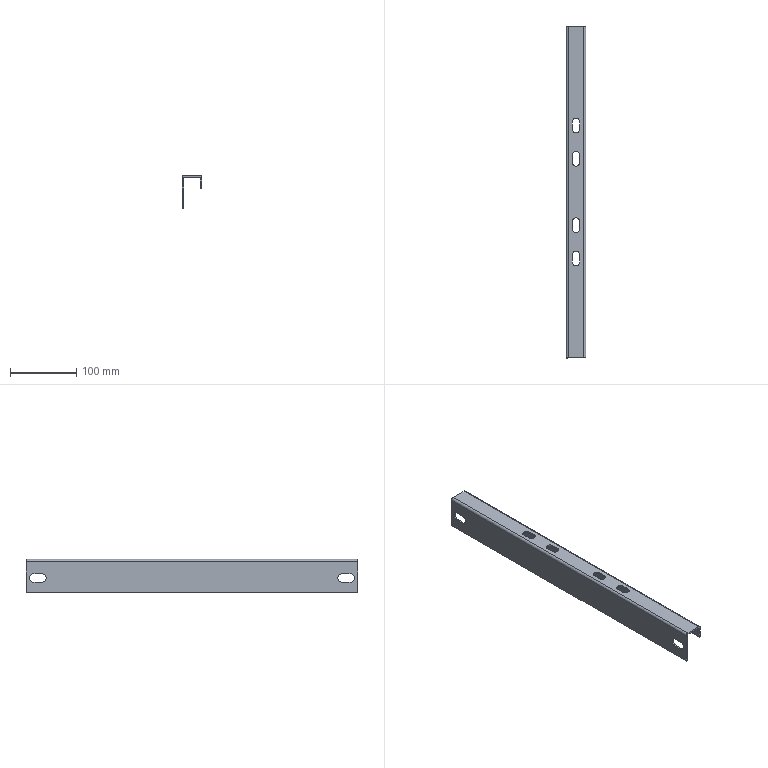Part | SolidWorks | features ICE 2, FlatPattern 1, SMBaseFlange 1, SheetMetal 1 | 1 solid | 46 faces | box 30 x 500 x 50 mm | volume 112732 mm3 | plane 30 | cylinder 16 | commonest cylinder face diameters 11 x8 13 x4 2 x2 7 x2
STEP:
#1=CARTESIAN_POINT('',(0.,250.,-3.5));
#2=VERTEX_POINT('',#1);
#3=CARTESIAN_POINT('',(2.5,250.,-3.5));
#4=VERTEX_POINT('',#3);
#5=CARTESIAN_POINT('',(0.,250.,-3.5));
#6=DIRECTION('',(1.,0.,0.));
#7=VECTOR('',#6,1000.);
#8=LINE('',#5,#7);
#9=EDGE_CURVE('',#2,#4,#8,.T.);
#10=ORIENTED_EDGE('',*,*,#9,.F.);
#11=CARTESIAN_POINT('',(3.5,250.,0.));
#12=VERTEX_POINT('',#11);
#13=CARTESIAN_POINT('',(3.5,250.,-3.5));
#14=DIRECTION('',(0.,1.,0.));
#15=DIRECTION('',(0.,0.,-1.));
#16=AXIS2_PLACEMENT_3D('',#13,#14,#15);
#17=CIRCLE('',#16,3.5);
#18=EDGE_CURVE('',#2,#12,#17,.T.);
#19=ORIENTED_EDGE('',*,*,#18,.T.);
#20=CARTESIAN_POINT('',(3.5,250.,-2.5));
#21=VERTEX_POINT('',#20);
#22=CARTESIAN_POINT('',(3.5,250.,-2.5));
#23=DIRECTION('',(0.,0.,1.));
#24=VECTOR('',#23,1000.);
#25=LINE('',#22,#24);
#26=EDGE_CURVE('',#21,#12,#25,.T.);
#27=ORIENTED_EDGE('',*,*,#26,.F.);
#28=CARTESIAN_POINT('',(3.5,250.,-3.5));
#29=DIRECTION('',(0.,1.,0.));
#30=DIRECTION('',(1.,0.,0.));
#31=AXIS2_PLACEMENT_3D('',#28,#29,#30);
#32=CIRCLE('',#31,1.);
#33=EDGE_CURVE('',#4,#21,#32,.T.);
#34=ORIENTED_EDGE('',*,*,#33,.F.);
#35=EDGE_LOOP('',(#10,#19,#27,#34));
#36=FACE_OUTER_BOUND('',#35,.T.);
#37=CARTESIAN_POINT('',(0.,250.,-3.5));
#38=DIRECTION('',(0.,1.,0.));
#39=DIRECTION('',(0.,0.,1.));
#40=AXIS2_PLACEMENT_3D('',#37,#38,#39);
#41=PLANE('',#40);
#42=ADVANCED_FACE('',(#36),#41,.T.);
#43=CARTESIAN_POINT('',(0.,250.,-50.));
#44=VERTEX_POINT('',#43);
#45=CARTESIAN_POINT('',(0.,250.,0.));
#46=DIRECTION('',(0.,0.,1.));
#47=VECTOR('',#46,1000.);
#48=LINE('',#45,#47);
#49=EDGE_CURVE('',#44,#2,#48,.T.);
#50=ORIENTED_EDGE('',*,*,#49,.T.);
#51=ORIENTED_EDGE('',*,*,#9,.T.);
#52=CARTESIAN_POINT('',(2.5,250.,-50.));
#53=VERTEX_POINT('',#52);
#54=CARTESIAN_POINT('',(2.5,250.,0.));
#55=DIRECTION('',(0.,0.,1.));
#56=VECTOR('',#55,1000.);
#57=LINE('',#54,#56);
#58=EDGE_CURVE('',#53,#4,#57,.T.);
#59=ORIENTED_EDGE('',*,*,#58,.F.);
#60=CARTESIAN_POINT('',(0.,250.,-50.));
#61=DIRECTION('',(1.,0.,0.));
#62=VECTOR('',#61,1000.);
#63=LINE('',#60,#62);
#64=EDGE_CURVE('',#44,#53,#63,.T.);
#65=ORIENTED_EDGE('',*,*,#64,.F.);
#66=EDGE_LOOP('',(#50,#51,#59,#65));
#67=FACE_OUTER_BOUND('',#66,.T.);
#68=CARTESIAN_POINT('',(3.5,250.,-2.5));
#69=DIRECTION('',(0.,1.,0.));
#70=DIRECTION('',(0.,0.,1.));
#71=AXIS2_PLACEMENT_3D('',#68,#69,#70);
#72=PLANE('',#71);
#73=ADVANCED_FACE('',(#67),#72,.T.);
#74=CARTESIAN_POINT('',(3.5,-250.,0.));
#75=VERTEX_POINT('',#74);
#76=CARTESIAN_POINT('',(3.5,-250.,-2.5));
#77=VERTEX_POINT('',#76);
#78=CARTESIAN_POINT('',(3.5,-250.,0.));
#79=DIRECTION('',(0.,0.,-1.));
#80=VECTOR('',#79,1000.);
#81=LINE('',#78,#80);
#82=EDGE_CURVE('',#75,#77,#81,.T.);
#83=ORIENTED_EDGE('',*,*,#82,.F.);
#84=CARTESIAN_POINT('',(0.,-250.,-3.5));
#85=VERTEX_POINT('',#84);
#86=CARTESIAN_POINT('',(3.5,-250.,-3.5));
#87=DIRECTION('',(0.,1.,0.));
#88=DIRECTION('',(0.,0.,-1.));
#89=AXIS2_PLACEMENT_3D('',#86,#87,#88);
#90=CIRCLE('',#89,3.5);
#91=EDGE_CURVE('',#85,#75,#90,.T.);
#92=ORIENTED_EDGE('',*,*,#91,.F.);
#93=CARTESIAN_POINT('',(2.5,-250.,-3.5));
#94=VERTEX_POINT('',#93);
#95=CARTESIAN_POINT('',(2.5,-250.,-3.5));
#96=DIRECTION('',(-1.,0.,0.));
#97=VECTOR('',#96,1000.);
#98=LINE('',#95,#97);
#99=EDGE_CURVE('',#94,#85,#98,.T.);
#100=ORIENTED_EDGE('',*,*,#99,.F.);
#101=CARTESIAN_POINT('',(3.5,-250.,-3.5));
#102=DIRECTION('',(0.,1.,0.));
#103=DIRECTION('',(1.,0.,0.));
#104=AXIS2_PLACEMENT_3D('',#101,#102,#103);
#105=CIRCLE('',#104,1.);
#106=EDGE_CURVE('',#94,#77,#105,.T.);
#107=ORIENTED_EDGE('',*,*,#106,.T.);
#108=EDGE_LOOP('',(#83,#92,#100,#107));
#109=FACE_OUTER_BOUND('',#108,.T.);
#110=CARTESIAN_POINT('',(3.5,-250.,0.));
#111=DIRECTION('',(0.,-1.,0.));
#112=DIRECTION('',(0.,0.,-1.));
#113=AXIS2_PLACEMENT_3D('',#110,#111,#112);
#114=PLANE('',#113);
#115=ADVANCED_FACE('',(#109),#114,.T.);
#116=CARTESIAN_POINT('',(26.5,-250.,0.));
#117=VERTEX_POINT('',#116);
#118=CARTESIAN_POINT('',(0.,-250.,0.));
#119=DIRECTION('',(1.,0.,0.));
#120=VECTOR('',#119,1000.);
#121=LINE('',#118,#120);
#122=EDGE_CURVE('',#75,#117,#121,.T.);
#123=ORIENTED_EDGE('',*,*,#122,.F.);
#124=ORIENTED_EDGE('',*,*,#82,.T.);
#125=CARTESIAN_POINT('',(26.5,-250.,-2.5));
#126=VERTEX_POINT('',#125);
#127=CARTESIAN_POINT('',(0.,-250.,-2.5));
#128=DIRECTION('',(1.,0.,0.));
#129=VECTOR('',#128,1000.);
#130=LINE('',#127,#129);
#131=EDGE_CURVE('',#77,#126,#130,.T.);
#132=ORIENTED_EDGE('',*,*,#131,.T.);
#133=CARTESIAN_POINT('',(26.5,-250.,-2.5));
#134=DIRECTION('',(0.,0.,1.));
#135=VECTOR('',#134,1000.);
#136=LINE('',#133,#135);
#137=EDGE_CURVE('',#126,#117,#136,.T.);
#138=ORIENTED_EDGE('',*,*,#137,.T.);
#139=EDGE_LOOP('',(#123,#124,#132,#138));
#140=FACE_OUTER_BOUND('',#139,.T.);
#141=CARTESIAN_POINT('',(2.5,-250.,-3.5));
#142=DIRECTION('',(0.,-1.,0.));
#143=DIRECTION('',(0.,0.,-1.));
#144=AXIS2_PLACEMENT_3D('',#141,#142,#143);
#145=PLANE('',#144);
#146=ADVANCED_FACE('',(#140),#145,.T.);
#147=CARTESIAN_POINT('',(26.5,250.,0.));
#148=VERTEX_POINT('',#147);
#149=CARTESIAN_POINT('',(26.5,250.,-2.5));
#150=VERTEX_POINT('',#149);
#151=CARTESIAN_POINT('',(26.5,250.,0.));
#152=DIRECTION('',(0.,0.,-1.));
#153=VECTOR('',#152,1000.);
#154=LINE('',#151,#153);
#155=EDGE_CURVE('',#148,#150,#154,.T.);
#156=ORIENTED_EDGE('',*,*,#155,.F.);
#157=CARTESIAN_POINT('',(30.,250.,-3.5));
#158=VERTEX_POINT('',#157);
#159=CARTESIAN_POINT('',(26.5,250.,-3.5));
#160=DIRECTION('',(0.,1.,0.));
#161=DIRECTION('',(0.,0.,-1.));
#162=AXIS2_PLACEMENT_3D('',#159,#160,#161);
#163=CIRCLE('',#162,3.5);
#164=EDGE_CURVE('',#148,#158,#163,.T.);
#165=ORIENTED_EDGE('',*,*,#164,.T.);
#166=CARTESIAN_POINT('',(27.5,250.,-3.5));
#167=VERTEX_POINT('',#166);
#168=CARTESIAN_POINT('',(27.5,250.,-3.5));
#169=DIRECTION('',(1.,0.,0.));
#170=VECTOR('',#169,1000.);
#171=LINE('',#168,#170);
#172=EDGE_CURVE('',#167,#158,#171,.T.);
#173=ORIENTED_EDGE('',*,*,#172,.F.);
#174=CARTESIAN_POINT('',(26.5,250.,-3.5));
#175=DIRECTION('',(0.,1.,0.));
#176=DIRECTION('',(1.,0.,0.));
#177=AXIS2_PLACEMENT_3D('',#174,#175,#176);
#178=CIRCLE('',#177,1.);
#179=EDGE_CURVE('',#150,#167,#178,.T.);
#180=ORIENTED_EDGE('',*,*,#179,.F.);
#181=EDGE_LOOP('',(#156,#165,#173,#180));
#182=FACE_OUTER_BOUND('',#181,.T.);
#183=CARTESIAN_POINT('',(26.5,250.,0.));
#184=DIRECTION('',(0.,1.,0.));
#185=DIRECTION('',(0.,0.,1.));
#186=AXIS2_PLACEMENT_3D('',#183,#184,#185);
#187=PLANE('',#186);
#188=ADVANCED_FACE('',(#182),#187,.T.);
#189=CARTESIAN_POINT('',(0.,250.,0.));
#190=DIRECTION('',(1.,0.,0.));
#191=VECTOR('',#190,1000.);
#192=LINE('',#189,#191);
#193=EDGE_CURVE('',#12,#148,#192,.T.);
#194=ORIENTED_EDGE('',*,*,#193,.T.);
#195=ORIENTED_EDGE('',*,*,#155,.T.);
#196=CARTESIAN_POINT('',(0.,250.,-2.5));
#197=DIRECTION('',(1.,0.,0.));
#198=VECTOR('',#197,1000.);
#199=LINE('',#196,#198);
#200=EDGE_CURVE('',#21,#150,#199,.T.);
#201=ORIENTED_EDGE('',*,*,#200,.F.);
#202=ORIENTED_EDGE('',*,*,#26,.T.);
#203=EDGE_LOOP('',(#194,#195,#201,#202));
#204=FACE_OUTER_BOUND('',#203,.T.);
#205=CARTESIAN_POINT('',(27.5,250.,-3.5));
#206=DIRECTION('',(0.,1.,0.));
#207=DIRECTION('',(0.,0.,1.));
#208=AXIS2_PLACEMENT_3D('',#205,#206,#207);
#209=PLANE('',#208);
#210=ADVANCED_FACE('',(#204),#209,.T.);
#211=CARTESIAN_POINT('',(30.,-250.,-3.5));
#212=VERTEX_POINT('',#211);
#213=CARTESIAN_POINT('',(27.5,-250.,-3.5));
#214=VERTEX_POINT('',#213);
#215=CARTESIAN_POINT('',(30.,-250.,-3.5));
#216=DIRECTION('',(-1.,0.,0.));
#217=VECTOR('',#216,1000.);
#218=LINE('',#215,#217);
#219=EDGE_CURVE('',#212,#214,#218,.T.);
#220=ORIENTED_EDGE('',*,*,#219,.F.);
#221=CARTESIAN_POINT('',(26.5,-250.,-3.5));
#222=DIRECTION('',(0.,1.,0.));
#223=DIRECTION('',(0.,0.,-1.));
#224=AXIS2_PLACEMENT_3D('',#221,#222,#223);
#225=CIRCLE('',#224,3.5);
#226=EDGE_CURVE('',#117,#212,#225,.T.);
#227=ORIENTED_EDGE('',*,*,#226,.F.);
#228=ORIENTED_EDGE('',*,*,#137,.F.);
#229=CARTESIAN_POINT('',(26.5,-250.,-3.5));
#230=DIRECTION('',(0.,1.,0.));
#231=DIRECTION('',(1.,0.,0.));
#232=AXIS2_PLACEMENT_3D('',#229,#230,#231);
#233=CIRCLE('',#232,1.);
#234=EDGE_CURVE('',#126,#214,#233,.T.);
#235=ORIENTED_EDGE('',*,*,#234,.T.);
#236=EDGE_LOOP('',(#220,#227,#228,#235));
#237=FACE_OUTER_BOUND('',#236,.T.);
#238=CARTESIAN_POINT('',(30.,-250.,-3.5));
#239=DIRECTION('',(0.,-1.,0.));
#240=DIRECTION('',(0.,0.,-1.));
#241=AXIS2_PLACEMENT_3D('',#238,#239,#240);
#242=PLANE('',#241);
#243=ADVANCED_FACE('',(#237),#242,.T.);
#244=CARTESIAN_POINT('',(30.,-250.,-20.));
#245=VERTEX_POINT('',#244);
#246=CARTESIAN_POINT('',(30.,-250.,0.));
#247=DIRECTION('',(0.,0.,-1.));
#248=VECTOR('',#247,1000.);
#249=LINE('',#246,#248);
#250=EDGE_CURVE('',#212,#245,#249,.T.);
#251=ORIENTED_EDGE('',*,*,#250,.F.);
#252=ORIENTED_EDGE('',*,*,#219,.T.);
#253=CARTESIAN_POINT('',(27.5,-250.,-20.));
#254=VERTEX_POINT('',#253);
#255=CARTESIAN_POINT('',(27.5,-250.,0.));
#256=DIRECTION('',(0.,0.,-1.));
#257=VECTOR('',#256,1000.);
#258=LINE('',#255,#257);
#259=EDGE_CURVE('',#214,#254,#258,.T.);
#260=ORIENTED_EDGE('',*,*,#259,.T.);
#261=CARTESIAN_POINT('',(27.5,-250.,-20.));
#262=DIRECTION('',(1.,0.,0.));
#263=VECTOR('',#262,1000.);
#264=LINE('',#261,#263);
#265=EDGE_CURVE('',#254,#245,#264,.T.);
#266=ORIENTED_EDGE('',*,*,#265,.T.);
#267=EDGE_LOOP('',(#251,#252,#260,#266));
#268=FACE_OUTER_BOUND('',#267,.T.);
#269=CARTESIAN_POINT('',(26.5,-250.,-2.5));
#270=DIRECTION('',(0.,-1.,0.));
#271=DIRECTION('',(0.,0.,-1.));
#272=AXIS2_PLACEMENT_3D('',#269,#270,#271);
#273=PLANE('',#272);
#274=ADVANCED_FACE('',(#268),#273,.T.);
#275=ORIENTED_EDGE('',*,*,#250,.T.);
#276=CARTESIAN_POINT('',(30.,250.,-20.));
#277=VERTEX_POINT('',#276);
#278=CARTESIAN_POINT('',(30.,250.,-20.));
#279=DIRECTION('',(0.,-1.,0.));
#280=VECTOR('',#279,1000.);
#281=LINE('',#278,#280);
#282=EDGE_CURVE('',#277,#245,#281,.T.);
#283=ORIENTED_EDGE('',*,*,#282,.F.);
#284=CARTESIAN_POINT('',(30.,250.,0.));
#285=DIRECTION('',(0.,0.,-1.));
#286=VECTOR('',#285,1000.);
#287=LINE('',#284,#286);
#288=EDGE_CURVE('',#158,#277,#287,.T.);
#289=ORIENTED_EDGE('',*,*,#288,.F.);
#290=CARTESIAN_POINT('',(30.,250.,-3.5));
#291=DIRECTION('',(0.,-1.,0.));
#292=VECTOR('',#291,1000.);
#293=LINE('',#290,#292);
#294=EDGE_CURVE('',#158,#212,#293,.T.);
#295=ORIENTED_EDGE('',*,*,#294,.T.);
#296=EDGE_LOOP('',(#275,#283,#289,#295));
#297=FACE_OUTER_BOUND('',#296,.T.);
#298=CARTESIAN_POINT('',(30.,250.,0.));
#299=DIRECTION('',(-1.,0.,0.));
#300=DIRECTION('',(0.,0.,1.));
#301=AXIS2_PLACEMENT_3D('',#298,#299,#300);
#302=PLANE('',#301);
#303=ADVANCED_FACE('',(#297),#302,.F.);
#304=ORIENTED_EDGE('',*,*,#265,.F.);
#305=CARTESIAN_POINT('',(27.5,250.,-20.));
#306=VERTEX_POINT('',#305);
#307=CARTESIAN_POINT('',(27.5,250.,-20.));
#308=DIRECTION('',(0.,-1.,0.));
#309=VECTOR('',#308,1000.);
#310=LINE('',#307,#309);
#311=EDGE_CURVE('',#306,#254,#310,.T.);
#312=ORIENTED_EDGE('',*,*,#311,.F.);
#313=CARTESIAN_POINT('',(27.5,250.,-20.));
#314=DIRECTION('',(1.,0.,0.));
#315=VECTOR('',#314,1000.);
#316=LINE('',#313,#315);
#317=EDGE_CURVE('',#306,#277,#316,.T.);
#318=ORIENTED_EDGE('',*,*,#317,.T.);
#319=ORIENTED_EDGE('',*,*,#282,.T.);
#320=EDGE_LOOP('',(#304,#312,#318,#319));
#321=FACE_OUTER_BOUND('',#320,.T.);
#322=CARTESIAN_POINT('',(27.5,250.,-20.));
#323=DIRECTION('',(0.,0.,-1.));
#324=DIRECTION('',(-1.,0.,0.));
#325=AXIS2_PLACEMENT_3D('',#322,#323,#324);
#326=PLANE('',#325);
#327=ADVANCED_FACE('',(#321),#326,.T.);
#328=ORIENTED_EDGE('',*,*,#259,.F.);
#329=CARTESIAN_POINT('',(27.5,250.,-3.5));
#330=DIRECTION('',(0.,-1.,0.));
#331=VECTOR('',#330,1000.);
#332=LINE('',#329,#331);
#333=EDGE_CURVE('',#167,#214,#332,.T.);
#334=ORIENTED_EDGE('',*,*,#333,.F.);
#335=CARTESIAN_POINT('',(27.5,250.,0.));
#336=DIRECTION('',(0.,0.,-1.));
#337=VECTOR('',#336,1000.);
#338=LINE('',#335,#337);
#339=EDGE_CURVE('',#167,#306,#338,.T.);
#340=ORIENTED_EDGE('',*,*,#339,.T.);
#341=ORIENTED_EDGE('',*,*,#311,.T.);
#342=EDGE_LOOP('',(#328,#334,#340,#341));
#343=FACE_OUTER_BOUND('',#342,.T.);
#344=CARTESIAN_POINT('',(27.5,250.,0.));
#345=DIRECTION('',(-1.,0.,0.));
#346=DIRECTION('',(0.,0.,1.));
#347=AXIS2_PLACEMENT_3D('',#344,#345,#346);
#348=PLANE('',#347);
#349=ADVANCED_FACE('',(#343),#348,.T.);
#350=ORIENTED_EDGE('',*,*,#234,.F.);
#351=CARTESIAN_POINT('',(26.5,250.,-2.5));
#352=DIRECTION('',(0.,-1.,0.));
#353=VECTOR('',#352,1000.);
#354=LINE('',#351,#353);
#355=EDGE_CURVE('',#150,#126,#354,.T.);
#356=ORIENTED_EDGE('',*,*,#355,.F.);
#357=ORIENTED_EDGE('',*,*,#179,.T.);
#358=ORIENTED_EDGE('',*,*,#333,.T.);
#359=EDGE_LOOP('',(#350,#356,#357,#358));
#360=FACE_OUTER_BOUND('',#359,.T.);
#361=CARTESIAN_POINT('',(26.5,250.,-3.5));
#362=DIRECTION('',(0.,-1.,0.));
#363=DIRECTION('',(0.,0.,-1.));
#364=AXIS2_PLACEMENT_3D('',#361,#362,#363);
#365=CYLINDRICAL_SURFACE('',#364,1.);
#366=ADVANCED_FACE('',(#360),#365,.F.);
#367=CARTESIAN_POINT('',(20.5,-105.5,-2.5));
#368=VERTEX_POINT('',#367);
#369=CARTESIAN_POINT('',(9.5,-105.5,-2.5));
#370=VERTEX_POINT('',#369);
#371=CARTESIAN_POINT('',(15.,-105.5,-2.5));
#372=DIRECTION('',(0.,0.,-1.));
#373=DIRECTION('',(-1.,0.,0.));
#374=AXIS2_PLACEMENT_3D('',#371,#372,#373);
#375=CIRCLE('',#374,5.5);
#376=EDGE_CURVE('',#368,#370,#375,.T.);
#377=ORIENTED_EDGE('',*,*,#376,.F.);
#378=CARTESIAN_POINT('',(20.5,-94.5,-2.5));
#379=VERTEX_POINT('',#378);
#380=CARTESIAN_POINT('',(20.5,-105.5,-2.5));
#381=DIRECTION('',(0.,-1.,0.));
#382=VECTOR('',#381,1000.);
#383=LINE('',#380,#382);
#384=EDGE_CURVE('',#379,#368,#383,.T.);
#385=ORIENTED_EDGE('',*,*,#384,.F.);
#386=CARTESIAN_POINT('',(9.5,-94.5,-2.5));
#387=VERTEX_POINT('',#386);
#388=CARTESIAN_POINT('',(15.,-94.5,-2.5));
#389=DIRECTION('',(0.,0.,-1.));
#390=DIRECTION('',(-1.,0.,0.));
#391=AXIS2_PLACEMENT_3D('',#388,#389,#390);
#392=CIRCLE('',#391,5.5);
#393=EDGE_CURVE('',#387,#379,#392,.T.);
#394=ORIENTED_EDGE('',*,*,#393,.F.);
#395=CARTESIAN_POINT('',(9.5,-105.5,-2.5));
#396=DIRECTION('',(0.,1.,0.));
#397=VECTOR('',#396,1000.);
#398=LINE('',#395,#397);
#399=EDGE_CURVE('',#370,#387,#398,.T.);
#400=ORIENTED_EDGE('',*,*,#399,.F.);
#401=EDGE_LOOP('',(#377,#385,#394,#400));
#402=FACE_BOUND('',#401,.T.);
#403=CARTESIAN_POINT('',(9.5,105.5,-2.5));
#404=VERTEX_POINT('',#403);
#405=CARTESIAN_POINT('',(20.5,105.5,-2.5));
#406=VERTEX_POINT('',#405);
#407=CARTESIAN_POINT('',(15.,105.5,-2.5));
#408=DIRECTION('',(0.,0.,-1.));
#409=DIRECTION('',(1.,0.,0.));
#410=AXIS2_PLACEMENT_3D('',#407,#408,#409);
#411=CIRCLE('',#410,5.5);
#412=EDGE_CURVE('',#404,#406,#411,.T.);
#413=ORIENTED_EDGE('',*,*,#412,.F.);
#414=CARTESIAN_POINT('',(9.5,94.5,-2.5));
#415=VERTEX_POINT('',#414);
#416=CARTESIAN_POINT('',(9.5,105.5,-2.5));
#417=DIRECTION('',(0.,1.,0.));
#418=VECTOR('',#417,1000.);
#419=LINE('',#416,#418);
#420=EDGE_CURVE('',#415,#404,#419,.T.);
#421=ORIENTED_EDGE('',*,*,#420,.F.);
#422=CARTESIAN_POINT('',(20.5,94.5,-2.5));
#423=VERTEX_POINT('',#422);
#424=CARTESIAN_POINT('',(15.,94.5,-2.5));
#425=DIRECTION('',(0.,0.,-1.));
#426=DIRECTION('',(1.,0.,0.));
#427=AXIS2_PLACEMENT_3D('',#424,#425,#426);
#428=CIRCLE('',#427,5.5);
#429=EDGE_CURVE('',#423,#415,#428,.T.);
#430=ORIENTED_EDGE('',*,*,#429,.F.);
#431=CARTESIAN_POINT('',(20.5,105.5,-2.5));
#432=DIRECTION('',(0.,-1.,0.));
#433=VECTOR('',#432,1000.);
#434=LINE('',#431,#433);
#435=EDGE_CURVE('',#406,#423,#434,.T.);
#436=ORIENTED_EDGE('',*,*,#435,.F.);
#437=EDGE_LOOP('',(#413,#421,#430,#436));
#438=FACE_BOUND('',#437,.T.);
#439=CARTESIAN_POINT('',(9.5,55.5,-2.5));
#440=VERTEX_POINT('',#439);
#441=CARTESIAN_POINT('',(20.5,55.5,-2.5));
#442=VERTEX_POINT('',#441);
#443=CARTESIAN_POINT('',(15.,55.5,-2.5));
#444=DIRECTION('',(0.,0.,-1.));
#445=DIRECTION('',(1.,0.,0.));
#446=AXIS2_PLACEMENT_3D('',#443,#444,#445);
#447=CIRCLE('',#446,5.5);
#448=EDGE_CURVE('',#440,#442,#447,.T.);
#449=ORIENTED_EDGE('',*,*,#448,.F.);
#450=CARTESIAN_POINT('',(9.5,44.5,-2.5));
#451=VERTEX_POINT('',#450);
#452=CARTESIAN_POINT('',(9.5,55.5,-2.5));
#453=DIRECTION('',(0.,1.,0.));
#454=VECTOR('',#453,1000.);
#455=LINE('',#452,#454);
#456=EDGE_CURVE('',#451,#440,#455,.T.);
#457=ORIENTED_EDGE('',*,*,#456,.F.);
#458=CARTESIAN_POINT('',(20.5,44.5,-2.5));
#459=VERTEX_POINT('',#458);
#460=CARTESIAN_POINT('',(15.,44.5,-2.5));
#461=DIRECTION('',(0.,0.,-1.));
#462=DIRECTION('',(1.,0.,0.));
#463=AXIS2_PLACEMENT_3D('',#460,#461,#462);
#464=CIRCLE('',#463,5.5);
#465=EDGE_CURVE('',#459,#451,#464,.T.);
#466=ORIENTED_EDGE('',*,*,#465,.F.);
#467=CARTESIAN_POINT('',(20.5,55.5,-2.5));
#468=DIRECTION('',(0.,-1.,0.));
#469=VECTOR('',#468,1000.);
#470=LINE('',#467,#469);
#471=EDGE_CURVE('',#442,#459,#470,.T.);
#472=ORIENTED_EDGE('',*,*,#471,.F.);
#473=EDGE_LOOP('',(#449,#457,#466,#472));
#474=FACE_BOUND('',#473,.T.);
#475=CARTESIAN_POINT('',(20.5,-55.5,-2.5));
#476=VERTEX_POINT('',#475);
#477=CARTESIAN_POINT('',(9.5,-55.5,-2.5));
#478=VERTEX_POINT('',#477);
#479=CARTESIAN_POINT('',(15.,-55.5,-2.5));
#480=DIRECTION('',(0.,0.,-1.));
#481=DIRECTION('',(-1.,0.,0.));
#482=AXIS2_PLACEMENT_3D('',#479,#480,#481);
#483=CIRCLE('',#482,5.5);
#484=EDGE_CURVE('',#476,#478,#483,.T.);
#485=ORIENTED_EDGE('',*,*,#484,.F.);
#486=CARTESIAN_POINT('',(20.5,-44.5,-2.5));
#487=VERTEX_POINT('',#486);
#488=CARTESIAN_POINT('',(20.5,-55.5,-2.5));
#489=DIRECTION('',(0.,-1.,0.));
#490=VECTOR('',#489,1000.);
#491=LINE('',#488,#490);
#492=EDGE_CURVE('',#487,#476,#491,.T.);
#493=ORIENTED_EDGE('',*,*,#492,.F.);
#494=CARTESIAN_POINT('',(9.5,-44.5,-2.5));
#495=VERTEX_POINT('',#494);
#496=CARTESIAN_POINT('',(15.,-44.5,-2.5));
#497=DIRECTION('',(0.,0.,-1.));
#498=DIRECTION('',(-1.,0.,0.));
#499=AXIS2_PLACEMENT_3D('',#496,#497,#498);
#500=CIRCLE('',#499,5.5);
#501=EDGE_CURVE('',#495,#487,#500,.T.);
#502=ORIENTED_EDGE('',*,*,#501,.F.);
#503=CARTESIAN_POINT('',(9.5,-55.5,-2.5));
#504=DIRECTION('',(0.,1.,0.));
#505=VECTOR('',#504,1000.);
#506=LINE('',#503,#505);
#507=EDGE_CURVE('',#478,#495,#506,.T.);
#508=ORIENTED_EDGE('',*,*,#507,.F.);
#509=EDGE_LOOP('',(#485,#493,#502,#508));
#510=FACE_BOUND('',#509,.T.);
#511=ORIENTED_EDGE('',*,*,#131,.F.);
#512=CARTESIAN_POINT('',(3.5,250.,-2.5));
#513=DIRECTION('',(0.,-1.,0.));
#514=VECTOR('',#513,1000.);
#515=LINE('',#512,#514);
#516=EDGE_CURVE('',#21,#77,#515,.T.);
#517=ORIENTED_EDGE('',*,*,#516,.F.);
#518=ORIENTED_EDGE('',*,*,#200,.T.);
#519=ORIENTED_EDGE('',*,*,#355,.T.);
#520=EDGE_LOOP('',(#511,#517,#518,#519));
#521=FACE_OUTER_BOUND('',#520,.T.);
#522=CARTESIAN_POINT('',(0.,250.,-2.5));
#523=DIRECTION('',(0.,0.,-1.));
#524=DIRECTION('',(-1.,0.,0.));
#525=AXIS2_PLACEMENT_3D('',#522,#523,#524);
#526=PLANE('',#525);
#527=ADVANCED_FACE('',(#402,#438,#474,#510,#521),#526,.T.);
#528=ORIENTED_EDGE('',*,*,#106,.F.);
#529=CARTESIAN_POINT('',(2.5,250.,-3.5));
#530=DIRECTION('',(0.,-1.,0.));
#531=VECTOR('',#530,1000.);
#532=LINE('',#529,#531);
#533=EDGE_CURVE('',#4,#94,#532,.T.);
#534=ORIENTED_EDGE('',*,*,#533,.F.);
#535=ORIENTED_EDGE('',*,*,#33,.T.);
#536=ORIENTED_EDGE('',*,*,#516,.T.);
#537=EDGE_LOOP('',(#528,#534,#535,#536));
#538=FACE_OUTER_BOUND('',#537,.T.);
#539=CARTESIAN_POINT('',(3.5,250.,-3.5));
#540=DIRECTION('',(0.,-1.,0.));
#541=DIRECTION('',(0.,0.,-1.));
#542=AXIS2_PLACEMENT_3D('',#539,#540,#541);
#543=CYLINDRICAL_SURFACE('',#542,1.);
#544=ADVANCED_FACE('',(#538),#543,.F.);
#545=CARTESIAN_POINT('',(2.5,-238.,-21.5));
#546=VERTEX_POINT('',#545);
#547=CARTESIAN_POINT('',(2.5,-238.,-34.5));
#548=VERTEX_POINT('',#547);
#549=CARTESIAN_POINT('',(2.5,-238.,-28.));
#550=DIRECTION('',(1.,0.,0.));
#551=DIRECTION('',(0.,0.,-1.));
#552=AXIS2_PLACEMENT_3D('',#549,#550,#551);
#553=CIRCLE('',#552,6.5);
#554=EDGE_CURVE('',#546,#548,#553,.T.);
#555=ORIENTED_EDGE('',*,*,#554,.F.);
#556=CARTESIAN_POINT('',(2.5,-226.,-21.5));
#557=VERTEX_POINT('',#556);
#558=CARTESIAN_POINT('',(2.5,250.,-21.5));
#559=DIRECTION('',(0.,-1.,0.));
#560=VECTOR('',#559,1000.);
#561=LINE('',#558,#560);
#562=EDGE_CURVE('',#557,#546,#561,.T.);
#563=ORIENTED_EDGE('',*,*,#562,.F.);
#564=CARTESIAN_POINT('',(2.5,-226.,-34.5));
#565=VERTEX_POINT('',#564);
#566=CARTESIAN_POINT('',(2.5,-226.,-28.));
#567=DIRECTION('',(1.,0.,0.));
#568=DIRECTION('',(0.,0.,-1.));
#569=AXIS2_PLACEMENT_3D('',#566,#567,#568);
#570=CIRCLE('',#569,6.5);
#571=EDGE_CURVE('',#565,#557,#570,.T.);
#572=ORIENTED_EDGE('',*,*,#571,.F.);
#573=CARTESIAN_POINT('',(2.5,250.,-34.5));
#574=DIRECTION('',(0.,1.,0.));
#575=VECTOR('',#574,1000.);
#576=LINE('',#573,#575);
#577=EDGE_CURVE('',#548,#565,#576,.T.);
#578=ORIENTED_EDGE('',*,*,#577,.F.);
#579=EDGE_LOOP('',(#555,#563,#572,#578));
#580=FACE_BOUND('',#579,.T.);
#581=CARTESIAN_POINT('',(2.5,238.,-34.5));
#582=VERTEX_POINT('',#581);
#583=CARTESIAN_POINT('',(2.5,238.,-21.5));
#584=VERTEX_POINT('',#583);
#585=CARTESIAN_POINT('',(2.5,238.,-28.));
#586=DIRECTION('',(1.,0.,0.));
#587=DIRECTION('',(0.,0.,-1.));
#588=AXIS2_PLACEMENT_3D('',#585,#586,#587);
#589=CIRCLE('',#588,6.5);
#590=EDGE_CURVE('',#582,#584,#589,.T.);
#591=ORIENTED_EDGE('',*,*,#590,.F.);
#592=CARTESIAN_POINT('',(2.5,226.,-34.5));
#593=VERTEX_POINT('',#592);
#594=CARTESIAN_POINT('',(2.5,250.,-34.5));
#595=DIRECTION('',(0.,1.,0.));
#596=VECTOR('',#595,1000.);
#597=LINE('',#594,#596);
#598=EDGE_CURVE('',#593,#582,#597,.T.);
#599=ORIENTED_EDGE('',*,*,#598,.F.);
#600=CARTESIAN_POINT('',(2.5,226.,-21.5));
#601=VERTEX_POINT('',#600);
#602=CARTESIAN_POINT('',(2.5,226.,-28.));
#603=DIRECTION('',(1.,0.,0.));
#604=DIRECTION('',(0.,0.,-1.));
#605=AXIS2_PLACEMENT_3D('',#602,#603,#604);
#606=CIRCLE('',#605,6.5);
#607=EDGE_CURVE('',#601,#593,#606,.T.);
#608=ORIENTED_EDGE('',*,*,#607,.F.);
#609=CARTESIAN_POINT('',(2.5,250.,-21.5));
#610=DIRECTION('',(0.,-1.,0.));
#611=VECTOR('',#610,1000.);
#612=LINE('',#609,#611);
#613=EDGE_CURVE('',#584,#601,#612,.T.);
#614=ORIENTED_EDGE('',*,*,#613,.F.);
#615=EDGE_LOOP('',(#591,#599,#608,#614));
#616=FACE_BOUND('',#615,.T.);
#617=CARTESIAN_POINT('',(2.5,-250.,-50.));
#618=VERTEX_POINT('',#617);
#619=CARTESIAN_POINT('',(2.5,-250.,0.));
#620=DIRECTION('',(0.,0.,1.));
#621=VECTOR('',#620,1000.);
#622=LINE('',#619,#621);
#623=EDGE_CURVE('',#618,#94,#622,.T.);
#624=ORIENTED_EDGE('',*,*,#623,.F.);
#625=CARTESIAN_POINT('',(2.5,250.,-50.));
#626=DIRECTION('',(0.,-1.,0.));
#627=VECTOR('',#626,1000.);
#628=LINE('',#625,#627);
#629=EDGE_CURVE('',#53,#618,#628,.T.);
#630=ORIENTED_EDGE('',*,*,#629,.F.);
#631=ORIENTED_EDGE('',*,*,#58,.T.);
#632=ORIENTED_EDGE('',*,*,#533,.T.);
#633=EDGE_LOOP('',(#624,#630,#631,#632));
#634=FACE_OUTER_BOUND('',#633,.T.);
#635=CARTESIAN_POINT('',(2.5,250.,0.));
#636=DIRECTION('',(1.,0.,0.));
#637=DIRECTION('',(0.,0.,-1.));
#638=AXIS2_PLACEMENT_3D('',#635,#636,#637);
#639=PLANE('',#638);
#640=ADVANCED_FACE('',(#580,#616,#634),#639,.T.);
#641=CARTESIAN_POINT('',(0.,-250.,-50.));
#642=VERTEX_POINT('',#641);
#643=CARTESIAN_POINT('',(0.,-250.,-50.));
#644=DIRECTION('',(1.,0.,0.));
#645=VECTOR('',#644,1000.);
#646=LINE('',#643,#645);
#647=EDGE_CURVE('',#642,#618,#646,.T.);
#648=ORIENTED_EDGE('',*,*,#647,.F.);
#649=CARTESIAN_POINT('',(0.,250.,-50.));
#650=DIRECTION('',(0.,-1.,0.));
#651=VECTOR('',#650,1000.);
#652=LINE('',#649,#651);
#653=EDGE_CURVE('',#44,#642,#652,.T.);
#654=ORIENTED_EDGE('',*,*,#653,.F.);
#655=ORIENTED_EDGE('',*,*,#64,.T.);
#656=ORIENTED_EDGE('',*,*,#629,.T.);
#657=EDGE_LOOP('',(#648,#654,#655,#656));
#658=FACE_OUTER_BOUND('',#657,.T.);
#659=CARTESIAN_POINT('',(0.,250.,-50.));
#660=DIRECTION('',(0.,0.,-1.));
#661=DIRECTION('',(-1.,0.,0.));
#662=AXIS2_PLACEMENT_3D('',#659,#660,#661);
#663=PLANE('',#662);
#664=ADVANCED_FACE('',(#658),#663,.T.);
#665=CARTESIAN_POINT('',(0.,-238.,-21.5));
#666=VERTEX_POINT('',#665);
#667=CARTESIAN_POINT('',(0.,-226.,-21.5));
#668=VERTEX_POINT('',#667);
#669=CARTESIAN_POINT('',(0.,-238.,-21.5));
#670=DIRECTION('',(0.,1.,0.));
#671=VECTOR('',#670,1000.);
#672=LINE('',#669,#671);
#673=EDGE_CURVE('',#666,#668,#672,.T.);
#674=ORIENTED_EDGE('',*,*,#673,.F.);
#675=CARTESIAN_POINT('',(0.,-238.,-34.5));
#676=VERTEX_POINT('',#675);
#677=CARTESIAN_POINT('',(0.,-238.,-28.));
#678=DIRECTION('',(-1.,0.,0.));
#679=DIRECTION('',(0.,0.,1.));
#680=AXIS2_PLACEMENT_3D('',#677,#678,#679);
#681=CIRCLE('',#680,6.5);
#682=EDGE_CURVE('',#676,#666,#681,.T.);
#683=ORIENTED_EDGE('',*,*,#682,.F.);
#684=CARTESIAN_POINT('',(0.,-226.,-34.5));
#685=VERTEX_POINT('',#684);
#686=CARTESIAN_POINT('',(0.,-238.,-34.5));
#687=DIRECTION('',(0.,-1.,0.));
#688=VECTOR('',#687,1000.);
#689=LINE('',#686,#688);
#690=EDGE_CURVE('',#685,#676,#689,.T.);
#691=ORIENTED_EDGE('',*,*,#690,.F.);
#692=CARTESIAN_POINT('',(0.,-226.,-28.));
#693=DIRECTION('',(-1.,0.,0.));
#694=DIRECTION('',(0.,0.,1.));
#695=AXIS2_PLACEMENT_3D('',#692,#693,#694);
#696=CIRCLE('',#695,6.5);
#697=EDGE_CURVE('',#668,#685,#696,.T.);
#698=ORIENTED_EDGE('',*,*,#697,.F.);
#699=EDGE_LOOP('',(#674,#683,#691,#698));
#700=FACE_BOUND('',#699,.T.);
#701=CARTESIAN_POINT('',(0.,238.,-34.5));
#702=VERTEX_POINT('',#701);
#703=CARTESIAN_POINT('',(0.,226.,-34.5));
#704=VERTEX_POINT('',#703);
#705=CARTESIAN_POINT('',(0.,238.,-34.5));
#706=DIRECTION('',(0.,-1.,0.));
#707=VECTOR('',#706,1000.);
#708=LINE('',#705,#707);
#709=EDGE_CURVE('',#702,#704,#708,.T.);
#710=ORIENTED_EDGE('',*,*,#709,.F.);
#711=CARTESIAN_POINT('',(0.,238.,-21.5));
#712=VERTEX_POINT('',#711);
#713=CARTESIAN_POINT('',(0.,238.,-28.));
#714=DIRECTION('',(-1.,0.,0.));
#715=DIRECTION('',(0.,0.,-1.));
#716=AXIS2_PLACEMENT_3D('',#713,#714,#715);
#717=CIRCLE('',#716,6.5);
#718=EDGE_CURVE('',#712,#702,#717,.T.);
#719=ORIENTED_EDGE('',*,*,#718,.F.);
#720=CARTESIAN_POINT('',(0.,226.,-21.5));
#721=VERTEX_POINT('',#720);
#722=CARTESIAN_POINT('',(0.,238.,-21.5));
#723=DIRECTION('',(0.,1.,0.));
#724=VECTOR('',#723,1000.);
#725=LINE('',#722,#724);
#726=EDGE_CURVE('',#721,#712,#725,.T.);
#727=ORIENTED_EDGE('',*,*,#726,.F.);
#728=CARTESIAN_POINT('',(0.,226.,-28.));
#729=DIRECTION('',(-1.,0.,0.));
#730=DIRECTION('',(0.,0.,-1.));
#731=AXIS2_PLACEMENT_3D('',#728,#729,#730);
#732=CIRCLE('',#731,6.5);
#733=EDGE_CURVE('',#704,#721,#732,.T.);
#734=ORIENTED_EDGE('',*,*,#733,.F.);
#735=EDGE_LOOP('',(#710,#719,#727,#734));
#736=FACE_BOUND('',#735,.T.);
#737=CARTESIAN_POINT('',(0.,-250.,0.));
#738=DIRECTION('',(0.,0.,1.));
#739=VECTOR('',#738,1000.);
#740=LINE('',#737,#739);
#741=EDGE_CURVE('',#642,#85,#740,.T.);
#742=ORIENTED_EDGE('',*,*,#741,.T.);
#743=CARTESIAN_POINT('',(0.,250.,-3.5));
#744=DIRECTION('',(0.,-1.,0.));
#745=VECTOR('',#744,1000.);
#746=LINE('',#743,#745);
#747=EDGE_CURVE('',#2,#85,#746,.T.);
#748=ORIENTED_EDGE('',*,*,#747,.F.);
#749=ORIENTED_EDGE('',*,*,#49,.F.);
#750=ORIENTED_EDGE('',*,*,#653,.T.);
#751=EDGE_LOOP('',(#742,#748,#749,#750));
#752=FACE_OUTER_BOUND('',#751,.T.);
#753=CARTESIAN_POINT('',(0.,250.,0.));
#754=DIRECTION('',(1.,0.,0.));
#755=DIRECTION('',(0.,0.,-1.));
#756=AXIS2_PLACEMENT_3D('',#753,#754,#755);
#757=PLANE('',#756);
#758=ADVANCED_FACE('',(#700,#736,#752),#757,.F.);
#759=ORIENTED_EDGE('',*,*,#91,.T.);
#760=CARTESIAN_POINT('',(3.5,250.,0.));
#761=DIRECTION('',(0.,-1.,0.));
#762=VECTOR('',#761,1000.);
#763=LINE('',#760,#762);
#764=EDGE_CURVE('',#12,#75,#763,.T.);
#765=ORIENTED_EDGE('',*,*,#764,.F.);
#766=ORIENTED_EDGE('',*,*,#18,.F.);
#767=ORIENTED_EDGE('',*,*,#747,.T.);
#768=EDGE_LOOP('',(#759,#765,#766,#767));
#769=FACE_OUTER_BOUND('',#768,.T.);
#770=CARTESIAN_POINT('',(3.5,250.,-3.5));
#771=DIRECTION('',(0.,-1.,0.));
#772=DIRECTION('',(0.,0.,-1.));
#773=AXIS2_PLACEMENT_3D('',#770,#771,#772);
#774=CYLINDRICAL_SURFACE('',#773,3.5);
#775=ADVANCED_FACE('',(#769),#774,.T.);
#776=CARTESIAN_POINT('',(20.5,-94.5,0.));
#777=VERTEX_POINT('',#776);
#778=CARTESIAN_POINT('',(20.5,-105.5,0.));
#779=VERTEX_POINT('',#778);
#780=CARTESIAN_POINT('',(20.5,250.,0.));
#781=DIRECTION('',(0.,-1.,0.));
#782=VECTOR('',#781,1000.);
#783=LINE('',#780,#782);
#784=EDGE_CURVE('',#777,#779,#783,.T.);
#785=ORIENTED_EDGE('',*,*,#784,.T.);
#786=CARTESIAN_POINT('',(9.5,-105.5,0.));
#787=VERTEX_POINT('',#786);
#788=CARTESIAN_POINT('',(15.,-105.5,0.));
#789=DIRECTION('',(0.,0.,-1.));
#790=DIRECTION('',(-1.,0.,0.));
#791=AXIS2_PLACEMENT_3D('',#788,#789,#790);
#792=CIRCLE('',#791,5.5);
#793=EDGE_CURVE('',#779,#787,#792,.T.);
#794=ORIENTED_EDGE('',*,*,#793,.T.);
#795=CARTESIAN_POINT('',(9.5,-94.5,0.));
#796=VERTEX_POINT('',#795);
#797=CARTESIAN_POINT('',(9.5,250.,0.));
#798=DIRECTION('',(0.,1.,0.));
#799=VECTOR('',#798,1000.);
#800=LINE('',#797,#799);
#801=EDGE_CURVE('',#787,#796,#800,.T.);
#802=ORIENTED_EDGE('',*,*,#801,.T.);
#803=CARTESIAN_POINT('',(15.,-94.5,0.));
#804=DIRECTION('',(0.,0.,-1.));
#805=DIRECTION('',(-1.,0.,0.));
#806=AXIS2_PLACEMENT_3D('',#803,#804,#805);
#807=CIRCLE('',#806,5.5);
#808=EDGE_CURVE('',#796,#777,#807,.T.);
#809=ORIENTED_EDGE('',*,*,#808,.T.);
#810=EDGE_LOOP('',(#785,#794,#802,#809));
#811=FACE_BOUND('',#810,.T.);
#812=CARTESIAN_POINT('',(9.5,94.5,0.));
#813=VERTEX_POINT('',#812);
#814=CARTESIAN_POINT('',(9.5,105.5,0.));
#815=VERTEX_POINT('',#814);
#816=CARTESIAN_POINT('',(9.5,250.,0.));
#817=DIRECTION('',(0.,1.,0.));
#818=VECTOR('',#817,1000.);
#819=LINE('',#816,#818);
#820=EDGE_CURVE('',#813,#815,#819,.T.);
#821=ORIENTED_EDGE('',*,*,#820,.T.);
#822=CARTESIAN_POINT('',(20.5,105.5,0.));
#823=VERTEX_POINT('',#822);
#824=CARTESIAN_POINT('',(15.,105.5,0.));
#825=DIRECTION('',(0.,0.,-1.));
#826=DIRECTION('',(-1.,0.,0.));
#827=AXIS2_PLACEMENT_3D('',#824,#825,#826);
#828=CIRCLE('',#827,5.5);
#829=EDGE_CURVE('',#815,#823,#828,.T.);
#830=ORIENTED_EDGE('',*,*,#829,.T.);
#831=CARTESIAN_POINT('',(20.5,94.5,0.));
#832=VERTEX_POINT('',#831);
#833=CARTESIAN_POINT('',(20.5,250.,0.));
#834=DIRECTION('',(0.,-1.,0.));
#835=VECTOR('',#834,1000.);
#836=LINE('',#833,#835);
#837=EDGE_CURVE('',#823,#832,#836,.T.);
#838=ORIENTED_EDGE('',*,*,#837,.T.);
#839=CARTESIAN_POINT('',(15.,94.5,0.));
#840=DIRECTION('',(0.,0.,-1.));
#841=DIRECTION('',(-1.,0.,0.));
#842=AXIS2_PLACEMENT_3D('',#839,#840,#841);
#843=CIRCLE('',#842,5.5);
#844=EDGE_CURVE('',#832,#813,#843,.T.);
#845=ORIENTED_EDGE('',*,*,#844,.T.);
#846=EDGE_LOOP('',(#821,#830,#838,#845));
#847=FACE_BOUND('',#846,.T.);
#848=CARTESIAN_POINT('',(9.5,44.5,0.));
#849=VERTEX_POINT('',#848);
#850=CARTESIAN_POINT('',(9.5,55.5,0.));
#851=VERTEX_POINT('',#850);
#852=CARTESIAN_POINT('',(9.5,250.,0.));
#853=DIRECTION('',(0.,1.,0.));
#854=VECTOR('',#853,1000.);
#855=LINE('',#852,#854);
#856=EDGE_CURVE('',#849,#851,#855,.T.);
#857=ORIENTED_EDGE('',*,*,#856,.T.);
#858=CARTESIAN_POINT('',(20.5,55.5,0.));
#859=VERTEX_POINT('',#858);
#860=CARTESIAN_POINT('',(15.,55.5,0.));
#861=DIRECTION('',(0.,0.,-1.));
#862=DIRECTION('',(-1.,0.,0.));
#863=AXIS2_PLACEMENT_3D('',#860,#861,#862);
#864=CIRCLE('',#863,5.5);
#865=EDGE_CURVE('',#851,#859,#864,.T.);
#866=ORIENTED_EDGE('',*,*,#865,.T.);
#867=CARTESIAN_POINT('',(20.5,44.5,0.));
#868=VERTEX_POINT('',#867);
#869=CARTESIAN_POINT('',(20.5,250.,0.));
#870=DIRECTION('',(0.,-1.,0.));
#871=VECTOR('',#870,1000.);
#872=LINE('',#869,#871);
#873=EDGE_CURVE('',#859,#868,#872,.T.);
#874=ORIENTED_EDGE('',*,*,#873,.T.);
#875=CARTESIAN_POINT('',(15.,44.5,0.));
#876=DIRECTION('',(0.,0.,-1.));
#877=DIRECTION('',(-1.,0.,0.));
#878=AXIS2_PLACEMENT_3D('',#875,#876,#877);
#879=CIRCLE('',#878,5.5);
#880=EDGE_CURVE('',#868,#849,#879,.T.);
#881=ORIENTED_EDGE('',*,*,#880,.T.);
#882=EDGE_LOOP('',(#857,#866,#874,#881));
#883=FACE_BOUND('',#882,.T.);
#884=CARTESIAN_POINT('',(20.5,-44.5,0.));
#885=VERTEX_POINT('',#884);
#886=CARTESIAN_POINT('',(20.5,-55.5,0.));
#887=VERTEX_POINT('',#886);
#888=CARTESIAN_POINT('',(20.5,250.,0.));
#889=DIRECTION('',(0.,-1.,0.));
#890=VECTOR('',#889,1000.);
#891=LINE('',#888,#890);
#892=EDGE_CURVE('',#885,#887,#891,.T.);
#893=ORIENTED_EDGE('',*,*,#892,.T.);
#894=CARTESIAN_POINT('',(9.5,-55.5,0.));
#895=VERTEX_POINT('',#894);
#896=CARTESIAN_POINT('',(15.,-55.5,0.));
#897=DIRECTION('',(0.,0.,-1.));
#898=DIRECTION('',(-1.,0.,0.));
#899=AXIS2_PLACEMENT_3D('',#896,#897,#898);
#900=CIRCLE('',#899,5.5);
#901=EDGE_CURVE('',#887,#895,#900,.T.);
#902=ORIENTED_EDGE('',*,*,#901,.T.);
#903=CARTESIAN_POINT('',(9.5,-44.5,0.));
#904=VERTEX_POINT('',#903);
#905=CARTESIAN_POINT('',(9.5,250.,0.));
#906=DIRECTION('',(0.,1.,0.));
#907=VECTOR('',#906,1000.);
#908=LINE('',#905,#907);
#909=EDGE_CURVE('',#895,#904,#908,.T.);
#910=ORIENTED_EDGE('',*,*,#909,.T.);
#911=CARTESIAN_POINT('',(15.,-44.5,0.));
#912=DIRECTION('',(0.,0.,-1.));
#913=DIRECTION('',(-1.,0.,0.));
#914=AXIS2_PLACEMENT_3D('',#911,#912,#913);
#915=CIRCLE('',#914,5.5);
#916=EDGE_CURVE('',#904,#885,#915,.T.);
#917=ORIENTED_EDGE('',*,*,#916,.T.);
#918=EDGE_LOOP('',(#893,#902,#910,#917));
#919=FACE_BOUND('',#918,.T.);
#920=ORIENTED_EDGE('',*,*,#122,.T.);
#921=CARTESIAN_POINT('',(26.5,250.,0.));
#922=DIRECTION('',(0.,-1.,0.));
#923=VECTOR('',#922,1000.);
#924=LINE('',#921,#923);
#925=EDGE_CURVE('',#148,#117,#924,.T.);
#926=ORIENTED_EDGE('',*,*,#925,.F.);
#927=ORIENTED_EDGE('',*,*,#193,.F.);
#928=ORIENTED_EDGE('',*,*,#764,.T.);
#929=EDGE_LOOP('',(#920,#926,#927,#928));
#930=FACE_OUTER_BOUND('',#929,.T.);
#931=CARTESIAN_POINT('',(0.,250.,0.));
#932=DIRECTION('',(0.,0.,-1.));
#933=DIRECTION('',(-1.,0.,0.));
#934=AXIS2_PLACEMENT_3D('',#931,#932,#933);
#935=PLANE('',#934);
#936=ADVANCED_FACE('',(#811,#847,#883,#919,#930),#935,.F.);
#937=ORIENTED_EDGE('',*,*,#226,.T.);
#938=ORIENTED_EDGE('',*,*,#294,.F.);
#939=ORIENTED_EDGE('',*,*,#164,.F.);
#940=ORIENTED_EDGE('',*,*,#925,.T.);
#941=EDGE_LOOP('',(#937,#938,#939,#940));
#942=FACE_OUTER_BOUND('',#941,.T.);
#943=CARTESIAN_POINT('',(26.5,250.,-3.5));
#944=DIRECTION('',(0.,-1.,0.));
#945=DIRECTION('',(0.,0.,-1.));
#946=AXIS2_PLACEMENT_3D('',#943,#944,#945);
#947=CYLINDRICAL_SURFACE('',#946,3.5);
#948=ADVANCED_FACE('',(#942),#947,.T.);
#949=ORIENTED_EDGE('',*,*,#288,.T.);
#950=ORIENTED_EDGE('',*,*,#317,.F.);
#951=ORIENTED_EDGE('',*,*,#339,.F.);
#952=ORIENTED_EDGE('',*,*,#172,.T.);
#953=EDGE_LOOP('',(#949,#950,#951,#952));
#954=FACE_OUTER_BOUND('',#953,.T.);
#955=CARTESIAN_POINT('',(26.5,250.,-3.5));
#956=DIRECTION('',(0.,1.,0.));
#957=DIRECTION('',(1.,0.,0.));
#958=AXIS2_PLACEMENT_3D('',#955,#956,#957);
#959=PLANE('',#958);
#960=ADVANCED_FACE('',(#954),#959,.T.);
#961=ORIENTED_EDGE('',*,*,#623,.T.);
#962=ORIENTED_EDGE('',*,*,#99,.T.);
#963=ORIENTED_EDGE('',*,*,#741,.F.);
#964=ORIENTED_EDGE('',*,*,#647,.T.);
#965=EDGE_LOOP('',(#961,#962,#963,#964));
#966=FACE_OUTER_BOUND('',#965,.T.);
#967=CARTESIAN_POINT('',(26.5,-250.,-3.5));
#968=DIRECTION('',(0.,1.,0.));
#969=DIRECTION('',(1.,0.,0.));
#970=AXIS2_PLACEMENT_3D('',#967,#968,#969);
#971=PLANE('',#970);
#972=ADVANCED_FACE('',(#966),#971,.F.);
#973=ORIENTED_EDGE('',*,*,#590,.T.);
#974=CARTESIAN_POINT('',(10.,238.,-21.5));
#975=DIRECTION('',(-1.,0.,0.));
#976=VECTOR('',#975,1000.);
#977=LINE('',#974,#976);
#978=EDGE_CURVE('',#584,#712,#977,.T.);
#979=ORIENTED_EDGE('',*,*,#978,.T.);
#980=ORIENTED_EDGE('',*,*,#718,.T.);
#981=CARTESIAN_POINT('',(10.,238.,-34.5));
#982=DIRECTION('',(-1.,0.,0.));
#983=VECTOR('',#982,1000.);
#984=LINE('',#981,#983);
#985=EDGE_CURVE('',#582,#702,#984,.T.);
#986=ORIENTED_EDGE('',*,*,#985,.F.);
#987=EDGE_LOOP('',(#973,#979,#980,#986));
#988=FACE_OUTER_BOUND('',#987,.T.);
#989=CARTESIAN_POINT('',(10.,238.,-28.));
#990=DIRECTION('',(-1.,0.,0.));
#991=DIRECTION('',(0.,0.,1.));
#992=AXIS2_PLACEMENT_3D('',#989,#990,#991);
#993=CYLINDRICAL_SURFACE('',#992,6.5);
#994=ADVANCED_FACE('',(#988),#993,.F.);
#995=ORIENTED_EDGE('',*,*,#613,.T.);
#996=CARTESIAN_POINT('',(10.,226.,-21.5));
#997=DIRECTION('',(-1.,0.,0.));
#998=VECTOR('',#997,1000.);
#999=LINE('',#996,#998);
#1000=EDGE_CURVE('',#601,#721,#999,.T.);
#1001=ORIENTED_EDGE('',*,*,#1000,.T.);
#1002=ORIENTED_EDGE('',*,*,#726,.T.);
#1003=ORIENTED_EDGE('',*,*,#978,.F.);
#1004=EDGE_LOOP('',(#995,#1001,#1002,#1003));
#1005=FACE_OUTER_BOUND('',#1004,.T.);
#1006=CARTESIAN_POINT('',(10.,238.,-21.5));
#1007=DIRECTION('',(0.,0.,1.));
#1008=DIRECTION('',(1.,0.,0.));
#1009=AXIS2_PLACEMENT_3D('',#1006,#1007,#1008);
#1010=PLANE('',#1009);
#1011=ADVANCED_FACE('',(#1005),#1010,.F.);
#1012=ORIENTED_EDGE('',*,*,#607,.T.);
#1013=CARTESIAN_POINT('',(10.,226.,-34.5));
#1014=DIRECTION('',(-1.,0.,0.));
#1015=VECTOR('',#1014,1000.);
#1016=LINE('',#1013,#1015);
#1017=EDGE_CURVE('',#593,#704,#1016,.T.);
#1018=ORIENTED_EDGE('',*,*,#1017,.T.);
#1019=ORIENTED_EDGE('',*,*,#733,.T.);
#1020=ORIENTED_EDGE('',*,*,#1000,.F.);
#1021=EDGE_LOOP('',(#1012,#1018,#1019,#1020));
#1022=FACE_OUTER_BOUND('',#1021,.T.);
#1023=CARTESIAN_POINT('',(10.,226.,-28.));
#1024=DIRECTION('',(-1.,0.,0.));
#1025=DIRECTION('',(0.,0.,1.));
#1026=AXIS2_PLACEMENT_3D('',#1023,#1024,#1025);
#1027=CYLINDRICAL_SURFACE('',#1026,6.5);
#1028=ADVANCED_FACE('',(#1022),#1027,.F.);
#1029=ORIENTED_EDGE('',*,*,#598,.T.);
#1030=ORIENTED_EDGE('',*,*,#985,.T.);
#1031=ORIENTED_EDGE('',*,*,#709,.T.);
#1032=ORIENTED_EDGE('',*,*,#1017,.F.);
#1033=EDGE_LOOP('',(#1029,#1030,#1031,#1032));
#1034=FACE_OUTER_BOUND('',#1033,.T.);
#1035=CARTESIAN_POINT('',(10.,238.,-34.5));
#1036=DIRECTION('',(0.,0.,-1.));
#1037=DIRECTION('',(-1.,0.,0.));
#1038=AXIS2_PLACEMENT_3D('',#1035,#1036,#1037);
#1039=PLANE('',#1038);
#1040=ADVANCED_FACE('',(#1034),#1039,.F.);
#1041=ORIENTED_EDGE('',*,*,#554,.T.);
#1042=CARTESIAN_POINT('',(10.,-238.,-34.5));
#1043=DIRECTION('',(-1.,0.,0.));
#1044=VECTOR('',#1043,1000.);
#1045=LINE('',#1042,#1044);
#1046=EDGE_CURVE('',#548,#676,#1045,.T.);
#1047=ORIENTED_EDGE('',*,*,#1046,.T.);
#1048=ORIENTED_EDGE('',*,*,#682,.T.);
#1049=CARTESIAN_POINT('',(10.,-238.,-21.5));
#1050=DIRECTION('',(-1.,0.,0.));
#1051=VECTOR('',#1050,1000.);
#1052=LINE('',#1049,#1051);
#1053=EDGE_CURVE('',#546,#666,#1052,.T.);
#1054=ORIENTED_EDGE('',*,*,#1053,.F.);
#1055=EDGE_LOOP('',(#1041,#1047,#1048,#1054));
#1056=FACE_OUTER_BOUND('',#1055,.T.);
#1057=CARTESIAN_POINT('',(10.,-238.,-28.));
#1058=DIRECTION('',(-1.,0.,0.));
#1059=DIRECTION('',(0.,0.,1.));
#1060=AXIS2_PLACEMENT_3D('',#1057,#1058,#1059);
#1061=CYLINDRICAL_SURFACE('',#1060,6.5);
#1062=ADVANCED_FACE('',(#1056),#1061,.F.);
#1063=ORIENTED_EDGE('',*,*,#577,.T.);
#1064=CARTESIAN_POINT('',(10.,-226.,-34.5));
#1065=DIRECTION('',(-1.,0.,0.));
#1066=VECTOR('',#1065,1000.);
#1067=LINE('',#1064,#1066);
#1068=EDGE_CURVE('',#565,#685,#1067,.T.);
#1069=ORIENTED_EDGE('',*,*,#1068,.T.);
#1070=ORIENTED_EDGE('',*,*,#690,.T.);
#1071=ORIENTED_EDGE('',*,*,#1046,.F.);
#1072=EDGE_LOOP('',(#1063,#1069,#1070,#1071));
#1073=FACE_OUTER_BOUND('',#1072,.T.);
#1074=CARTESIAN_POINT('',(10.,-238.,-34.5));
#1075=DIRECTION('',(0.,0.,-1.));
#1076=DIRECTION('',(-1.,0.,0.));
#1077=AXIS2_PLACEMENT_3D('',#1074,#1075,#1076);
#1078=PLANE('',#1077);
#1079=ADVANCED_FACE('',(#1073),#1078,.F.);
#1080=ORIENTED_EDGE('',*,*,#571,.T.);
#1081=CARTESIAN_POINT('',(10.,-226.,-21.5));
#1082=DIRECTION('',(-1.,0.,0.));
#1083=VECTOR('',#1082,1000.);
#1084=LINE('',#1081,#1083);
#1085=EDGE_CURVE('',#557,#668,#1084,.T.);
#1086=ORIENTED_EDGE('',*,*,#1085,.T.);
#1087=ORIENTED_EDGE('',*,*,#697,.T.);
#1088=ORIENTED_EDGE('',*,*,#1068,.F.);
#1089=EDGE_LOOP('',(#1080,#1086,#1087,#1088));
#1090=FACE_OUTER_BOUND('',#1089,.T.);
#1091=CARTESIAN_POINT('',(10.,-226.,-28.));
#1092=DIRECTION('',(-1.,0.,0.));
#1093=DIRECTION('',(0.,0.,1.));
#1094=AXIS2_PLACEMENT_3D('',#1091,#1092,#1093);
#1095=CYLINDRICAL_SURFACE('',#1094,6.5);
#1096=ADVANCED_FACE('',(#1090),#1095,.F.);
#1097=ORIENTED_EDGE('',*,*,#562,.T.);
#1098=ORIENTED_EDGE('',*,*,#1053,.T.);
#1099=ORIENTED_EDGE('',*,*,#673,.T.);
#1100=ORIENTED_EDGE('',*,*,#1085,.F.);
#1101=EDGE_LOOP('',(#1097,#1098,#1099,#1100));
#1102=FACE_OUTER_BOUND('',#1101,.T.);
#1103=CARTESIAN_POINT('',(10.,-238.,-21.5));
#1104=DIRECTION('',(0.,0.,1.));
#1105=DIRECTION('',(0.,-1.,0.));
#1106=AXIS2_PLACEMENT_3D('',#1103,#1104,#1105);
#1107=PLANE('',#1106);
#1108=ADVANCED_FACE('',(#1102),#1107,.F.);
#1109=CARTESIAN_POINT('',(20.5,-55.5,7.5));
#1110=DIRECTION('',(0.,0.,-1.));
#1111=VECTOR('',#1110,1000.);
#1112=LINE('',#1109,#1111);
#1113=EDGE_CURVE('',#887,#476,#1112,.T.);
#1114=ORIENTED_EDGE('',*,*,#1113,.T.);
#1115=ORIENTED_EDGE('',*,*,#484,.T.);
#1116=CARTESIAN_POINT('',(9.5,-55.5,7.5));
#1117=DIRECTION('',(0.,0.,-1.));
#1118=VECTOR('',#1117,1000.);
#1119=LINE('',#1116,#1118);
#1120=EDGE_CURVE('',#895,#478,#1119,.T.);
#1121=ORIENTED_EDGE('',*,*,#1120,.F.);
#1122=ORIENTED_EDGE('',*,*,#901,.F.);
#1123=EDGE_LOOP('',(#1114,#1115,#1121,#1122));
#1124=FACE_OUTER_BOUND('',#1123,.T.);
#1125=CARTESIAN_POINT('',(15.,-55.5,7.5));
#1126=DIRECTION('',(0.,0.,-1.));
#1127=DIRECTION('',(-1.,0.,0.));
#1128=AXIS2_PLACEMENT_3D('',#1125,#1126,#1127);
#1129=CYLINDRICAL_SURFACE('',#1128,5.5);
#1130=ADVANCED_FACE('',(#1124),#1129,.F.);
#1131=CARTESIAN_POINT('',(20.5,-44.5,7.5));
#1132=DIRECTION('',(0.,0.,-1.));
#1133=VECTOR('',#1132,1000.);
#1134=LINE('',#1131,#1133);
#1135=EDGE_CURVE('',#885,#487,#1134,.T.);
#1136=ORIENTED_EDGE('',*,*,#1135,.T.);
#1137=ORIENTED_EDGE('',*,*,#492,.T.);
#1138=ORIENTED_EDGE('',*,*,#1113,.F.);
#1139=ORIENTED_EDGE('',*,*,#892,.F.);
#1140=EDGE_LOOP('',(#1136,#1137,#1138,#1139));
#1141=FACE_OUTER_BOUND('',#1140,.T.);
#1142=CARTESIAN_POINT('',(20.5,-55.5,7.5));
#1143=DIRECTION('',(1.,0.,0.));
#1144=DIRECTION('',(0.,0.,-1.));
#1145=AXIS2_PLACEMENT_3D('',#1142,#1143,#1144);
#1146=PLANE('',#1145);
#1147=ADVANCED_FACE('',(#1141),#1146,.F.);
#1148=CARTESIAN_POINT('',(9.5,-44.5,7.5));
#1149=DIRECTION('',(0.,0.,-1.));
#1150=VECTOR('',#1149,1000.);
#1151=LINE('',#1148,#1150);
#1152=EDGE_CURVE('',#904,#495,#1151,.T.);
#1153=ORIENTED_EDGE('',*,*,#1152,.T.);
#1154=ORIENTED_EDGE('',*,*,#501,.T.);
#1155=ORIENTED_EDGE('',*,*,#1135,.F.);
#1156=ORIENTED_EDGE('',*,*,#916,.F.);
#1157=EDGE_LOOP('',(#1153,#1154,#1155,#1156));
#1158=FACE_OUTER_BOUND('',#1157,.T.);
#1159=CARTESIAN_POINT('',(15.,-44.5,7.5));
#1160=DIRECTION('',(0.,0.,-1.));
#1161=DIRECTION('',(-1.,0.,0.));
#1162=AXIS2_PLACEMENT_3D('',#1159,#1160,#1161);
#1163=CYLINDRICAL_SURFACE('',#1162,5.5);
#1164=ADVANCED_FACE('',(#1158),#1163,.F.);
#1165=ORIENTED_EDGE('',*,*,#1120,.T.);
#1166=ORIENTED_EDGE('',*,*,#507,.T.);
#1167=ORIENTED_EDGE('',*,*,#1152,.F.);
#1168=ORIENTED_EDGE('',*,*,#909,.F.);
#1169=EDGE_LOOP('',(#1165,#1166,#1167,#1168));
#1170=FACE_OUTER_BOUND('',#1169,.T.);
#1171=CARTESIAN_POINT('',(9.5,-55.5,7.5));
#1172=DIRECTION('',(-1.,0.,0.));
#1173=DIRECTION('',(0.,-1.,0.));
#1174=AXIS2_PLACEMENT_3D('',#1171,#1172,#1173);
#1175=PLANE('',#1174);
#1176=ADVANCED_FACE('',(#1170),#1175,.F.);
#1177=CARTESIAN_POINT('',(9.5,55.5,7.5));
#1178=DIRECTION('',(0.,0.,-1.));
#1179=VECTOR('',#1178,1000.);
#1180=LINE('',#1177,#1179);
#1181=EDGE_CURVE('',#851,#440,#1180,.T.);
#1182=ORIENTED_EDGE('',*,*,#1181,.T.);
#1183=ORIENTED_EDGE('',*,*,#448,.T.);
#1184=CARTESIAN_POINT('',(20.5,55.5,7.5));
#1185=DIRECTION('',(0.,0.,-1.));
#1186=VECTOR('',#1185,1000.);
#1187=LINE('',#1184,#1186);
#1188=EDGE_CURVE('',#859,#442,#1187,.T.);
#1189=ORIENTED_EDGE('',*,*,#1188,.F.);
#1190=ORIENTED_EDGE('',*,*,#865,.F.);
#1191=EDGE_LOOP('',(#1182,#1183,#1189,#1190));
#1192=FACE_OUTER_BOUND('',#1191,.T.);
#1193=CARTESIAN_POINT('',(15.,55.5,7.5));
#1194=DIRECTION('',(0.,0.,-1.));
#1195=DIRECTION('',(-1.,0.,0.));
#1196=AXIS2_PLACEMENT_3D('',#1193,#1194,#1195);
#1197=CYLINDRICAL_SURFACE('',#1196,5.5);
#1198=ADVANCED_FACE('',(#1192),#1197,.F.);
#1199=CARTESIAN_POINT('',(9.5,44.5,7.5));
#1200=DIRECTION('',(0.,0.,-1.));
#1201=VECTOR('',#1200,1000.);
#1202=LINE('',#1199,#1201);
#1203=EDGE_CURVE('',#849,#451,#1202,.T.);
#1204=ORIENTED_EDGE('',*,*,#1203,.T.);
#1205=ORIENTED_EDGE('',*,*,#456,.T.);
#1206=ORIENTED_EDGE('',*,*,#1181,.F.);
#1207=ORIENTED_EDGE('',*,*,#856,.F.);
#1208=EDGE_LOOP('',(#1204,#1205,#1206,#1207));
#1209=FACE_OUTER_BOUND('',#1208,.T.);
#1210=CARTESIAN_POINT('',(9.5,55.5,7.5));
#1211=DIRECTION('',(-1.,0.,0.));
#1212=DIRECTION('',(0.,0.,1.));
#1213=AXIS2_PLACEMENT_3D('',#1210,#1211,#1212);
#1214=PLANE('',#1213);
#1215=ADVANCED_FACE('',(#1209),#1214,.F.);
#1216=CARTESIAN_POINT('',(20.5,44.5,7.5));
#1217=DIRECTION('',(0.,0.,-1.));
#1218=VECTOR('',#1217,1000.);
#1219=LINE('',#1216,#1218);
#1220=EDGE_CURVE('',#868,#459,#1219,.T.);
#1221=ORIENTED_EDGE('',*,*,#1220,.T.);
#1222=ORIENTED_EDGE('',*,*,#465,.T.);
#1223=ORIENTED_EDGE('',*,*,#1203,.F.);
#1224=ORIENTED_EDGE('',*,*,#880,.F.);
#1225=EDGE_LOOP('',(#1221,#1222,#1223,#1224));
#1226=FACE_OUTER_BOUND('',#1225,.T.);
#1227=CARTESIAN_POINT('',(15.,44.5,7.5));
#1228=DIRECTION('',(0.,0.,-1.));
#1229=DIRECTION('',(-1.,0.,0.));
#1230=AXIS2_PLACEMENT_3D('',#1227,#1228,#1229);
#1231=CYLINDRICAL_SURFACE('',#1230,5.5);
#1232=ADVANCED_FACE('',(#1226),#1231,.F.);
#1233=ORIENTED_EDGE('',*,*,#1188,.T.);
#1234=ORIENTED_EDGE('',*,*,#471,.T.);
#1235=ORIENTED_EDGE('',*,*,#1220,.F.);
#1236=ORIENTED_EDGE('',*,*,#873,.F.);
#1237=EDGE_LOOP('',(#1233,#1234,#1235,#1236));
#1238=FACE_OUTER_BOUND('',#1237,.T.);
#1239=CARTESIAN_POINT('',(20.5,55.5,7.5));
#1240=DIRECTION('',(1.,0.,0.));
#1241=DIRECTION('',(0.,0.,-1.));
#1242=AXIS2_PLACEMENT_3D('',#1239,#1240,#1241);
#1243=PLANE('',#1242);
#1244=ADVANCED_FACE('',(#1238),#1243,.F.);
#1245=CARTESIAN_POINT('',(9.5,105.5,7.5));
#1246=DIRECTION('',(0.,0.,-1.));
#1247=VECTOR('',#1246,1000.);
#1248=LINE('',#1245,#1247);
#1249=EDGE_CURVE('',#815,#404,#1248,.T.);
#1250=ORIENTED_EDGE('',*,*,#1249,.T.);
#1251=ORIENTED_EDGE('',*,*,#412,.T.);
#1252=CARTESIAN_POINT('',(20.5,105.5,7.5));
#1253=DIRECTION('',(0.,0.,-1.));
#1254=VECTOR('',#1253,1000.);
#1255=LINE('',#1252,#1254);
#1256=EDGE_CURVE('',#823,#406,#1255,.T.);
#1257=ORIENTED_EDGE('',*,*,#1256,.F.);
#1258=ORIENTED_EDGE('',*,*,#829,.F.);
#1259=EDGE_LOOP('',(#1250,#1251,#1257,#1258));
#1260=FACE_OUTER_BOUND('',#1259,.T.);
#1261=CARTESIAN_POINT('',(15.,105.5,7.5));
#1262=DIRECTION('',(0.,0.,-1.));
#1263=DIRECTION('',(-1.,0.,0.));
#1264=AXIS2_PLACEMENT_3D('',#1261,#1262,#1263);
#1265=CYLINDRICAL_SURFACE('',#1264,5.5);
#1266=ADVANCED_FACE('',(#1260),#1265,.F.);
#1267=CARTESIAN_POINT('',(9.5,94.5,7.5));
#1268=DIRECTION('',(0.,0.,-1.));
#1269=VECTOR('',#1268,1000.);
#1270=LINE('',#1267,#1269);
#1271=EDGE_CURVE('',#813,#415,#1270,.T.);
#1272=ORIENTED_EDGE('',*,*,#1271,.T.);
#1273=ORIENTED_EDGE('',*,*,#420,.T.);
#1274=ORIENTED_EDGE('',*,*,#1249,.F.);
#1275=ORIENTED_EDGE('',*,*,#820,.F.);
#1276=EDGE_LOOP('',(#1272,#1273,#1274,#1275));
#1277=FACE_OUTER_BOUND('',#1276,.T.);
#1278=CARTESIAN_POINT('',(9.5,105.5,7.5));
#1279=DIRECTION('',(-1.,0.,0.));
#1280=DIRECTION('',(0.,-1.,0.));
#1281=AXIS2_PLACEMENT_3D('',#1278,#1279,#1280);
#1282=PLANE('',#1281);
#1283=ADVANCED_FACE('',(#1277),#1282,.F.);
#1284=CARTESIAN_POINT('',(20.5,94.5,7.5));
#1285=DIRECTION('',(0.,0.,-1.));
#1286=VECTOR('',#1285,1000.);
#1287=LINE('',#1284,#1286);
#1288=EDGE_CURVE('',#832,#423,#1287,.T.);
#1289=ORIENTED_EDGE('',*,*,#1288,.T.);
#1290=ORIENTED_EDGE('',*,*,#429,.T.);
#1291=ORIENTED_EDGE('',*,*,#1271,.F.);
#1292=ORIENTED_EDGE('',*,*,#844,.F.);
#1293=EDGE_LOOP('',(#1289,#1290,#1291,#1292));
#1294=FACE_OUTER_BOUND('',#1293,.T.);
#1295=CARTESIAN_POINT('',(15.,94.5,7.5));
#1296=DIRECTION('',(0.,0.,-1.));
#1297=DIRECTION('',(-1.,0.,0.));
#1298=AXIS2_PLACEMENT_3D('',#1295,#1296,#1297);
#1299=CYLINDRICAL_SURFACE('',#1298,5.5);
#1300=ADVANCED_FACE('',(#1294),#1299,.F.);
#1301=ORIENTED_EDGE('',*,*,#1256,.T.);
#1302=ORIENTED_EDGE('',*,*,#435,.T.);
#1303=ORIENTED_EDGE('',*,*,#1288,.F.);
#1304=ORIENTED_EDGE('',*,*,#837,.F.);
#1305=EDGE_LOOP('',(#1301,#1302,#1303,#1304));
#1306=FACE_OUTER_BOUND('',#1305,.T.);
#1307=CARTESIAN_POINT('',(20.5,105.5,7.5));
#1308=DIRECTION('',(1.,0.,0.));
#1309=DIRECTION('',(0.,0.,-1.));
#1310=AXIS2_PLACEMENT_3D('',#1307,#1308,#1309);
#1311=PLANE('',#1310);
#1312=ADVANCED_FACE('',(#1306),#1311,.F.);
#1313=CARTESIAN_POINT('',(20.5,-105.5,7.5));
#1314=DIRECTION('',(0.,0.,-1.));
#1315=VECTOR('',#1314,1000.);
#1316=LINE('',#1313,#1315);
#1317=EDGE_CURVE('',#779,#368,#1316,.T.);
#1318=ORIENTED_EDGE('',*,*,#1317,.T.);
#1319=ORIENTED_EDGE('',*,*,#376,.T.);
#1320=CARTESIAN_POINT('',(9.5,-105.5,7.5));
#1321=DIRECTION('',(0.,0.,-1.));
#1322=VECTOR('',#1321,1000.);
#1323=LINE('',#1320,#1322);
#1324=EDGE_CURVE('',#787,#370,#1323,.T.);
#1325=ORIENTED_EDGE('',*,*,#1324,.F.);
#1326=ORIENTED_EDGE('',*,*,#793,.F.);
#1327=EDGE_LOOP('',(#1318,#1319,#1325,#1326));
#1328=FACE_OUTER_BOUND('',#1327,.T.);
#1329=CARTESIAN_POINT('',(15.,-105.5,7.5));
#1330=DIRECTION('',(0.,0.,-1.));
#1331=DIRECTION('',(-1.,0.,0.));
#1332=AXIS2_PLACEMENT_3D('',#1329,#1330,#1331);
#1333=CYLINDRICAL_SURFACE('',#1332,5.5);
#1334=ADVANCED_FACE('',(#1328),#1333,.F.);
#1335=CARTESIAN_POINT('',(20.5,-94.5,7.5));
#1336=DIRECTION('',(0.,0.,-1.));
#1337=VECTOR('',#1336,1000.);
#1338=LINE('',#1335,#1337);
#1339=EDGE_CURVE('',#777,#379,#1338,.T.);
#1340=ORIENTED_EDGE('',*,*,#1339,.T.);
#1341=ORIENTED_EDGE('',*,*,#384,.T.);
#1342=ORIENTED_EDGE('',*,*,#1317,.F.);
#1343=ORIENTED_EDGE('',*,*,#784,.F.);
#1344=EDGE_LOOP('',(#1340,#1341,#1342,#1343));
#1345=FACE_OUTER_BOUND('',#1344,.T.);
#1346=CARTESIAN_POINT('',(20.5,-105.5,7.5));
#1347=DIRECTION('',(1.,0.,0.));
#1348=DIRECTION('',(0.,0.,-1.));
#1349=AXIS2_PLACEMENT_3D('',#1346,#1347,#1348);
#1350=PLANE('',#1349);
#1351=ADVANCED_FACE('',(#1345),#1350,.F.);
#1352=CARTESIAN_POINT('',(9.5,-94.5,7.5));
#1353=DIRECTION('',(0.,0.,-1.));
#1354=VECTOR('',#1353,1000.);
#1355=LINE('',#1352,#1354);
#1356=EDGE_CURVE('',#796,#387,#1355,.T.);
#1357=ORIENTED_EDGE('',*,*,#1356,.T.);
#1358=ORIENTED_EDGE('',*,*,#393,.T.);
#1359=ORIENTED_EDGE('',*,*,#1339,.F.);
#1360=ORIENTED_EDGE('',*,*,#808,.F.);
#1361=EDGE_LOOP('',(#1357,#1358,#1359,#1360));
#1362=FACE_OUTER_BOUND('',#1361,.T.);
#1363=CARTESIAN_POINT('',(15.,-94.5,7.5));
#1364=DIRECTION('',(0.,0.,-1.));
#1365=DIRECTION('',(-1.,0.,0.));
#1366=AXIS2_PLACEMENT_3D('',#1363,#1364,#1365);
#1367=CYLINDRICAL_SURFACE('',#1366,5.5);
#1368=ADVANCED_FACE('',(#1362),#1367,.F.);
#1369=ORIENTED_EDGE('',*,*,#1324,.T.);
#1370=ORIENTED_EDGE('',*,*,#399,.T.);
#1371=ORIENTED_EDGE('',*,*,#1356,.F.);
#1372=ORIENTED_EDGE('',*,*,#801,.F.);
#1373=EDGE_LOOP('',(#1369,#1370,#1371,#1372));
#1374=FACE_OUTER_BOUND('',#1373,.T.);
#1375=CARTESIAN_POINT('',(9.5,-105.5,7.5));
#1376=DIRECTION('',(-1.,0.,0.));
#1377=DIRECTION('',(0.,0.,1.));
#1378=AXIS2_PLACEMENT_3D('',#1375,#1376,#1377);
#1379=PLANE('',#1378);
#1380=ADVANCED_FACE('',(#1374),#1379,.F.);
#1381=CLOSED_SHELL('',(#42,#73,#115,#146,#188,#210,#243,#274,#303,#327,#349,#366,#527,#544,#640,#664,#758,#775,#936,#948,#960,#972,#994,#1011,#1028,#1040,#1062,#1079,#1096,#1108,#1130,#1147,#1164,#1176,#1198,#1215,#1232,#1244,#1266,#1283,#1300,#1312,#1334,#1351,#1368,#1380));
#1382=MANIFOLD_SOLID_BREP('',#1381);
#1383=CARTESIAN_POINT('',(0.,0.,0.));
#1384=DIRECTION('',(0.,0.,1.));
#1385=DIRECTION('',(1.,0.,0.));
#1386=AXIS2_PLACEMENT_3D('',#1383,#1384,#1385);
#1387=(LENGTH_UNIT()NAMED_UNIT(*)SI_UNIT(.MILLI.,.METRE.));
#1388=UNCERTAINTY_MEASURE_WITH_UNIT(LENGTH_MEASURE(0.00001),#1387,'','');
#1389=(NAMED_UNIT(*)PLANE_ANGLE_UNIT()SI_UNIT($,.RADIAN.));
#1390=(NAMED_UNIT(*)SI_UNIT($,.STERADIAN.)SOLID_ANGLE_UNIT());
#1391=(GEOMETRIC_REPRESENTATION_CONTEXT(3)GLOBAL_UNCERTAINTY_ASSIGNED_CONTEXT((#1388))GLOBAL_UNIT_ASSIGNED_CONTEXT((#1387,#1389,#1390))REPRESENTATION_CONTEXT('',''));
#1392=ADVANCED_BREP_SHAPE_REPRESENTATION('',(#1382,#1386),#1391);